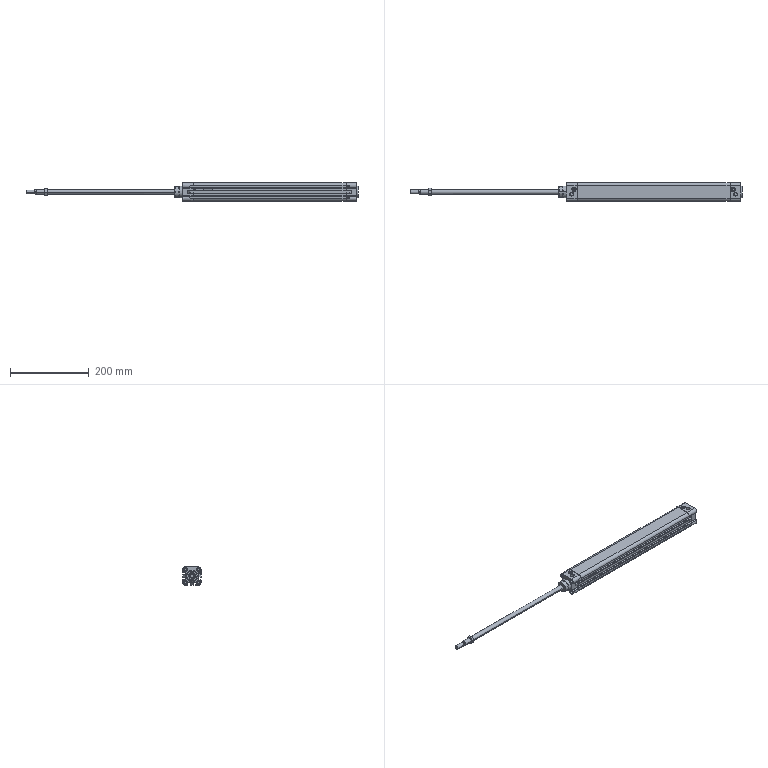Part | SolidWorks | 4 solids | 477 faces | box 845 x 46.8 x 46.5 mm | volume 590487 mm3 | plane 212 | cylinder 202 | cone 61 | spline 2 | commonest cylinder face diameters 1 x90 4.917 x16 9.4 x16 8 x12 14 x10 15 x10